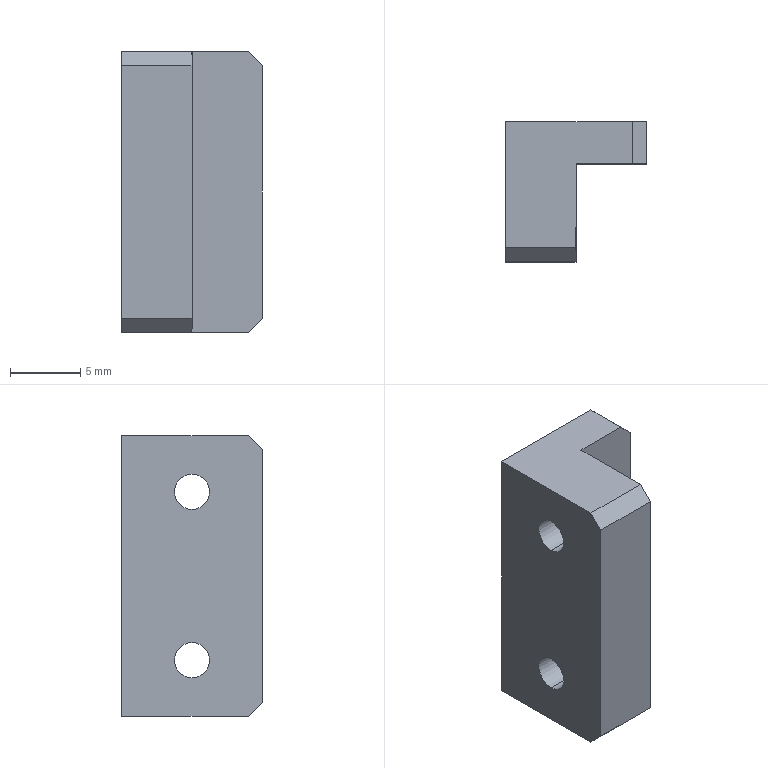Part | STEP file | FBDS-TL-002 | 1 solid | 16 faces | box 10 x 10 x 20 mm | volume 1243 mm3 | plane 12 | cylinder 4 | commonest cylinder face diameters 2.5 x4
STEP:
#1=CARTESIAN_POINT('',(5.,-5.,2.75));
#2=VERTEX_POINT('',#1);
#3=CARTESIAN_POINT('',(5.,-5.,5.25));
#4=VERTEX_POINT('',#3);
#5=CARTESIAN_POINT('',(5.,-5.,4.));
#6=DIRECTION('',(-1.,0.,0.));
#7=DIRECTION('',(0.,0.,1.));
#8=AXIS2_PLACEMENT_3D('',#5,#6,#7);
#9=CIRCLE('',#8,1.25);
#10=EDGE_CURVE('',#2,#4,#9,.T.);
#11=ORIENTED_EDGE('',*,*,#10,.F.);
#12=CARTESIAN_POINT('',(0.,-5.,2.75));
#13=VERTEX_POINT('',#12);
#14=CARTESIAN_POINT('',(0.,-5.,2.75));
#15=DIRECTION('',(-1.,0.,0.));
#16=VECTOR('',#15,1000.);
#17=LINE('',#14,#16);
#18=EDGE_CURVE('',#2,#13,#17,.T.);
#19=ORIENTED_EDGE('',*,*,#18,.T.);
#20=CARTESIAN_POINT('',(0.,-5.,5.25));
#21=VERTEX_POINT('',#20);
#22=CARTESIAN_POINT('',(0.,-5.,4.));
#23=DIRECTION('',(-1.,0.,0.));
#24=DIRECTION('',(0.,0.,1.));
#25=AXIS2_PLACEMENT_3D('',#22,#23,#24);
#26=CIRCLE('',#25,1.25);
#27=EDGE_CURVE('',#13,#21,#26,.T.);
#28=ORIENTED_EDGE('',*,*,#27,.T.);
#29=CARTESIAN_POINT('',(0.,-5.,5.25));
#30=DIRECTION('',(-1.,0.,0.));
#31=VECTOR('',#30,1000.);
#32=LINE('',#29,#31);
#33=EDGE_CURVE('',#4,#21,#32,.T.);
#34=ORIENTED_EDGE('',*,*,#33,.F.);
#35=EDGE_LOOP('',(#11,#19,#28,#34));
#36=FACE_OUTER_BOUND('',#35,.T.);
#37=CARTESIAN_POINT('',(0.,-5.,4.));
#38=DIRECTION('',(-1.,0.,0.));
#39=DIRECTION('',(0.,0.,1.));
#40=AXIS2_PLACEMENT_3D('',#37,#38,#39);
#41=CYLINDRICAL_SURFACE('',#40,1.25);
#42=ADVANCED_FACE('',(#36),#41,.F.);
#43=CARTESIAN_POINT('',(5.,-5.,14.75));
#44=VERTEX_POINT('',#43);
#45=CARTESIAN_POINT('',(5.,-5.,17.25));
#46=VERTEX_POINT('',#45);
#47=CARTESIAN_POINT('',(5.,-5.,16.));
#48=DIRECTION('',(-1.,0.,0.));
#49=DIRECTION('',(0.,0.,1.));
#50=AXIS2_PLACEMENT_3D('',#47,#48,#49);
#51=CIRCLE('',#50,1.25);
#52=EDGE_CURVE('',#44,#46,#51,.T.);
#53=ORIENTED_EDGE('',*,*,#52,.F.);
#54=CARTESIAN_POINT('',(0.,-5.,14.75));
#55=VERTEX_POINT('',#54);
#56=CARTESIAN_POINT('',(0.,-5.,14.75));
#57=DIRECTION('',(-1.,0.,0.));
#58=VECTOR('',#57,1000.);
#59=LINE('',#56,#58);
#60=EDGE_CURVE('',#44,#55,#59,.T.);
#61=ORIENTED_EDGE('',*,*,#60,.T.);
#62=CARTESIAN_POINT('',(0.,-5.,17.25));
#63=VERTEX_POINT('',#62);
#64=CARTESIAN_POINT('',(0.,-5.,16.));
#65=DIRECTION('',(-1.,0.,0.));
#66=DIRECTION('',(0.,0.,1.));
#67=AXIS2_PLACEMENT_3D('',#64,#65,#66);
#68=CIRCLE('',#67,1.25);
#69=EDGE_CURVE('',#55,#63,#68,.T.);
#70=ORIENTED_EDGE('',*,*,#69,.T.);
#71=CARTESIAN_POINT('',(0.,-5.,17.25));
#72=DIRECTION('',(-1.,0.,0.));
#73=VECTOR('',#72,1000.);
#74=LINE('',#71,#73);
#75=EDGE_CURVE('',#46,#63,#74,.T.);
#76=ORIENTED_EDGE('',*,*,#75,.F.);
#77=EDGE_LOOP('',(#53,#61,#70,#76));
#78=FACE_OUTER_BOUND('',#77,.T.);
#79=CARTESIAN_POINT('',(0.,-5.,16.));
#80=DIRECTION('',(-1.,0.,0.));
#81=DIRECTION('',(0.,0.,1.));
#82=AXIS2_PLACEMENT_3D('',#79,#80,#81);
#83=CYLINDRICAL_SURFACE('',#82,1.25);
#84=ADVANCED_FACE('',(#78),#83,.F.);
#85=CARTESIAN_POINT('',(0.,-5.,4.));
#86=DIRECTION('',(-1.,0.,0.));
#87=DIRECTION('',(0.,0.,1.));
#88=AXIS2_PLACEMENT_3D('',#85,#86,#87);
#89=CIRCLE('',#88,1.25);
#90=EDGE_CURVE('',#21,#13,#89,.T.);
#91=ORIENTED_EDGE('',*,*,#90,.F.);
#92=ORIENTED_EDGE('',*,*,#27,.F.);
#93=EDGE_LOOP('',(#91,#92));
#94=FACE_BOUND('',#93,.T.);
#95=CARTESIAN_POINT('',(0.,-5.,16.));
#96=DIRECTION('',(-1.,0.,0.));
#97=DIRECTION('',(0.,0.,1.));
#98=AXIS2_PLACEMENT_3D('',#95,#96,#97);
#99=CIRCLE('',#98,1.25);
#100=EDGE_CURVE('',#63,#55,#99,.T.);
#101=ORIENTED_EDGE('',*,*,#100,.F.);
#102=ORIENTED_EDGE('',*,*,#69,.F.);
#103=EDGE_LOOP('',(#101,#102));
#104=FACE_BOUND('',#103,.T.);
#105=CARTESIAN_POINT('',(0.,0.,0.));
#106=VERTEX_POINT('',#105);
#107=CARTESIAN_POINT('',(0.,-9.,0.));
#108=VERTEX_POINT('',#107);
#109=CARTESIAN_POINT('',(0.,-10.,0.));
#110=DIRECTION('',(0.,-1.,0.));
#111=VECTOR('',#110,1000.);
#112=LINE('',#109,#111);
#113=EDGE_CURVE('',#106,#108,#112,.T.);
#114=ORIENTED_EDGE('',*,*,#113,.T.);
#115=CARTESIAN_POINT('',(0.,-10.,1.));
#116=VERTEX_POINT('',#115);
#117=CARTESIAN_POINT('',(0.,-10.,1.));
#118=DIRECTION('',(0.,-0.7071,0.7071));
#119=VECTOR('',#118,1000.);
#120=LINE('',#117,#119);
#121=EDGE_CURVE('',#108,#116,#120,.T.);
#122=ORIENTED_EDGE('',*,*,#121,.T.);
#123=CARTESIAN_POINT('',(0.,-10.,19.));
#124=VERTEX_POINT('',#123);
#125=CARTESIAN_POINT('',(0.,-10.,20.));
#126=DIRECTION('',(0.,0.,-1.));
#127=VECTOR('',#126,1000.);
#128=LINE('',#125,#127);
#129=EDGE_CURVE('',#124,#116,#128,.T.);
#130=ORIENTED_EDGE('',*,*,#129,.F.);
#131=CARTESIAN_POINT('',(0.,-9.,20.));
#132=VERTEX_POINT('',#131);
#133=CARTESIAN_POINT('',(0.,-9.,20.));
#134=DIRECTION('',(0.,0.7071,0.7071));
#135=VECTOR('',#134,1000.);
#136=LINE('',#133,#135);
#137=EDGE_CURVE('',#124,#132,#136,.T.);
#138=ORIENTED_EDGE('',*,*,#137,.T.);
#139=CARTESIAN_POINT('',(0.,0.,20.));
#140=VERTEX_POINT('',#139);
#141=CARTESIAN_POINT('',(0.,-10.,20.));
#142=DIRECTION('',(0.,-1.,0.));
#143=VECTOR('',#142,1000.);
#144=LINE('',#141,#143);
#145=EDGE_CURVE('',#140,#132,#144,.T.);
#146=ORIENTED_EDGE('',*,*,#145,.F.);
#147=CARTESIAN_POINT('',(0.,0.,20.));
#148=DIRECTION('',(0.,0.,-1.));
#149=VECTOR('',#148,1000.);
#150=LINE('',#147,#149);
#151=EDGE_CURVE('',#140,#106,#150,.T.);
#152=ORIENTED_EDGE('',*,*,#151,.T.);
#153=EDGE_LOOP('',(#114,#122,#130,#138,#146,#152));
#154=FACE_OUTER_BOUND('',#153,.T.);
#155=CARTESIAN_POINT('',(0.,-10.,20.));
#156=DIRECTION('',(1.,0.,0.));
#157=DIRECTION('',(0.,0.,-1.));
#158=AXIS2_PLACEMENT_3D('',#155,#156,#157);
#159=PLANE('',#158);
#160=ADVANCED_FACE('',(#94,#104,#154),#159,.F.);
#161=ORIENTED_EDGE('',*,*,#129,.T.);
#162=CARTESIAN_POINT('',(5.,-10.,1.));
#163=VERTEX_POINT('',#162);
#164=CARTESIAN_POINT('',(5.,-10.,1.));
#165=DIRECTION('',(1.,0.,0.));
#166=VECTOR('',#165,1000.);
#167=LINE('',#164,#166);
#168=EDGE_CURVE('',#116,#163,#167,.T.);
#169=ORIENTED_EDGE('',*,*,#168,.T.);
#170=CARTESIAN_POINT('',(5.,-10.,19.));
#171=VERTEX_POINT('',#170);
#172=CARTESIAN_POINT('',(5.,-10.,20.));
#173=DIRECTION('',(0.,0.,-1.));
#174=VECTOR('',#173,1000.);
#175=LINE('',#172,#174);
#176=EDGE_CURVE('',#171,#163,#175,.T.);
#177=ORIENTED_EDGE('',*,*,#176,.F.);
#178=CARTESIAN_POINT('',(5.,-10.,19.));
#179=DIRECTION('',(-1.,0.,0.));
#180=VECTOR('',#179,1000.);
#181=LINE('',#178,#180);
#182=EDGE_CURVE('',#171,#124,#181,.T.);
#183=ORIENTED_EDGE('',*,*,#182,.T.);
#184=EDGE_LOOP('',(#161,#169,#177,#183));
#185=FACE_OUTER_BOUND('',#184,.T.);
#186=CARTESIAN_POINT('',(5.,-10.,20.));
#187=DIRECTION('',(0.,1.,0.));
#188=DIRECTION('',(-1.,0.,0.));
#189=AXIS2_PLACEMENT_3D('',#186,#187,#188);
#190=PLANE('',#189);
#191=ADVANCED_FACE('',(#185),#190,.F.);
#192=CARTESIAN_POINT('',(5.,-5.,4.));
#193=DIRECTION('',(-1.,0.,0.));
#194=DIRECTION('',(0.,0.,1.));
#195=AXIS2_PLACEMENT_3D('',#192,#193,#194);
#196=CIRCLE('',#195,1.25);
#197=EDGE_CURVE('',#4,#2,#196,.T.);
#198=ORIENTED_EDGE('',*,*,#197,.T.);
#199=ORIENTED_EDGE('',*,*,#10,.T.);
#200=EDGE_LOOP('',(#198,#199));
#201=FACE_BOUND('',#200,.T.);
#202=CARTESIAN_POINT('',(5.,-5.,16.));
#203=DIRECTION('',(-1.,0.,0.));
#204=DIRECTION('',(0.,0.,1.));
#205=AXIS2_PLACEMENT_3D('',#202,#203,#204);
#206=CIRCLE('',#205,1.25);
#207=EDGE_CURVE('',#46,#44,#206,.T.);
#208=ORIENTED_EDGE('',*,*,#207,.T.);
#209=ORIENTED_EDGE('',*,*,#52,.T.);
#210=EDGE_LOOP('',(#208,#209));
#211=FACE_BOUND('',#210,.T.);
#212=ORIENTED_EDGE('',*,*,#176,.T.);
#213=CARTESIAN_POINT('',(5.,-9.,0.));
#214=VERTEX_POINT('',#213);
#215=CARTESIAN_POINT('',(5.,-10.,1.));
#216=DIRECTION('',(0.,0.7071,-0.7071));
#217=VECTOR('',#216,1000.);
#218=LINE('',#215,#217);
#219=EDGE_CURVE('',#163,#214,#218,.T.);
#220=ORIENTED_EDGE('',*,*,#219,.T.);
#221=CARTESIAN_POINT('',(5.,-3.,0.));
#222=VERTEX_POINT('',#221);
#223=CARTESIAN_POINT('',(5.,-3.,0.));
#224=DIRECTION('',(0.,1.,0.));
#225=VECTOR('',#224,1000.);
#226=LINE('',#223,#225);
#227=EDGE_CURVE('',#214,#222,#226,.T.);
#228=ORIENTED_EDGE('',*,*,#227,.T.);
#229=CARTESIAN_POINT('',(5.,-3.,20.));
#230=VERTEX_POINT('',#229);
#231=CARTESIAN_POINT('',(5.,-3.,20.));
#232=DIRECTION('',(0.,0.,-1.));
#233=VECTOR('',#232,1000.);
#234=LINE('',#231,#233);
#235=EDGE_CURVE('',#230,#222,#234,.T.);
#236=ORIENTED_EDGE('',*,*,#235,.F.);
#237=CARTESIAN_POINT('',(5.,-9.,20.));
#238=VERTEX_POINT('',#237);
#239=CARTESIAN_POINT('',(5.,-3.,20.));
#240=DIRECTION('',(0.,1.,0.));
#241=VECTOR('',#240,1000.);
#242=LINE('',#239,#241);
#243=EDGE_CURVE('',#238,#230,#242,.T.);
#244=ORIENTED_EDGE('',*,*,#243,.F.);
#245=CARTESIAN_POINT('',(5.,-9.,20.));
#246=DIRECTION('',(0.,-0.7071,-0.7071));
#247=VECTOR('',#246,1000.);
#248=LINE('',#245,#247);
#249=EDGE_CURVE('',#238,#171,#248,.T.);
#250=ORIENTED_EDGE('',*,*,#249,.T.);
#251=EDGE_LOOP('',(#212,#220,#228,#236,#244,#250));
#252=FACE_OUTER_BOUND('',#251,.T.);
#253=CARTESIAN_POINT('',(5.,-3.,20.));
#254=DIRECTION('',(-1.,0.,0.));
#255=DIRECTION('',(0.,0.,1.));
#256=AXIS2_PLACEMENT_3D('',#253,#254,#255);
#257=PLANE('',#256);
#258=ADVANCED_FACE('',(#201,#211,#252),#257,.F.);
#259=CARTESIAN_POINT('',(9.,-3.,0.));
#260=VERTEX_POINT('',#259);
#261=CARTESIAN_POINT('',(10.,-3.,0.));
#262=DIRECTION('',(1.,0.,0.));
#263=VECTOR('',#262,1000.);
#264=LINE('',#261,#263);
#265=EDGE_CURVE('',#222,#260,#264,.T.);
#266=ORIENTED_EDGE('',*,*,#265,.T.);
#267=CARTESIAN_POINT('',(10.,-3.,1.));
#268=VERTEX_POINT('',#267);
#269=CARTESIAN_POINT('',(10.,-3.,1.));
#270=DIRECTION('',(0.7071,0.,0.7071));
#271=VECTOR('',#270,1000.);
#272=LINE('',#269,#271);
#273=EDGE_CURVE('',#260,#268,#272,.T.);
#274=ORIENTED_EDGE('',*,*,#273,.T.);
#275=CARTESIAN_POINT('',(10.,-3.,19.));
#276=VERTEX_POINT('',#275);
#277=CARTESIAN_POINT('',(10.,-3.,20.));
#278=DIRECTION('',(0.,0.,-1.));
#279=VECTOR('',#278,1000.);
#280=LINE('',#277,#279);
#281=EDGE_CURVE('',#276,#268,#280,.T.);
#282=ORIENTED_EDGE('',*,*,#281,.F.);
#283=CARTESIAN_POINT('',(9.,-3.,20.));
#284=VERTEX_POINT('',#283);
#285=CARTESIAN_POINT('',(9.,-3.,20.));
#286=DIRECTION('',(-0.7071,0.,0.7071));
#287=VECTOR('',#286,1000.);
#288=LINE('',#285,#287);
#289=EDGE_CURVE('',#276,#284,#288,.T.);
#290=ORIENTED_EDGE('',*,*,#289,.T.);
#291=CARTESIAN_POINT('',(10.,-3.,20.));
#292=DIRECTION('',(1.,0.,0.));
#293=VECTOR('',#292,1000.);
#294=LINE('',#291,#293);
#295=EDGE_CURVE('',#230,#284,#294,.T.);
#296=ORIENTED_EDGE('',*,*,#295,.F.);
#297=ORIENTED_EDGE('',*,*,#235,.T.);
#298=EDGE_LOOP('',(#266,#274,#282,#290,#296,#297));
#299=FACE_OUTER_BOUND('',#298,.T.);
#300=CARTESIAN_POINT('',(10.,-3.,20.));
#301=DIRECTION('',(0.,1.,0.));
#302=DIRECTION('',(-1.,0.,0.));
#303=AXIS2_PLACEMENT_3D('',#300,#301,#302);
#304=PLANE('',#303);
#305=ADVANCED_FACE('',(#299),#304,.F.);
#306=ORIENTED_EDGE('',*,*,#281,.T.);
#307=CARTESIAN_POINT('',(10.,0.,1.));
#308=VERTEX_POINT('',#307);
#309=CARTESIAN_POINT('',(10.,0.,1.));
#310=DIRECTION('',(0.,1.,0.));
#311=VECTOR('',#310,1000.);
#312=LINE('',#309,#311);
#313=EDGE_CURVE('',#268,#308,#312,.T.);
#314=ORIENTED_EDGE('',*,*,#313,.T.);
#315=CARTESIAN_POINT('',(10.,0.,19.));
#316=VERTEX_POINT('',#315);
#317=CARTESIAN_POINT('',(10.,0.,20.));
#318=DIRECTION('',(0.,0.,-1.));
#319=VECTOR('',#318,1000.);
#320=LINE('',#317,#319);
#321=EDGE_CURVE('',#316,#308,#320,.T.);
#322=ORIENTED_EDGE('',*,*,#321,.F.);
#323=CARTESIAN_POINT('',(10.,0.,19.));
#324=DIRECTION('',(0.,-1.,0.));
#325=VECTOR('',#324,1000.);
#326=LINE('',#323,#325);
#327=EDGE_CURVE('',#316,#276,#326,.T.);
#328=ORIENTED_EDGE('',*,*,#327,.T.);
#329=EDGE_LOOP('',(#306,#314,#322,#328));
#330=FACE_OUTER_BOUND('',#329,.T.);
#331=CARTESIAN_POINT('',(10.,0.,20.));
#332=DIRECTION('',(-1.,0.,0.));
#333=DIRECTION('',(0.,0.,1.));
#334=AXIS2_PLACEMENT_3D('',#331,#332,#333);
#335=PLANE('',#334);
#336=ADVANCED_FACE('',(#330),#335,.F.);
#337=ORIENTED_EDGE('',*,*,#321,.T.);
#338=CARTESIAN_POINT('',(9.,0.,0.));
#339=VERTEX_POINT('',#338);
#340=CARTESIAN_POINT('',(10.,0.,1.));
#341=DIRECTION('',(-0.7071,0.,-0.7071));
#342=VECTOR('',#341,1000.);
#343=LINE('',#340,#342);
#344=EDGE_CURVE('',#308,#339,#343,.T.);
#345=ORIENTED_EDGE('',*,*,#344,.T.);
#346=CARTESIAN_POINT('',(0.,0.,0.));
#347=DIRECTION('',(-1.,0.,0.));
#348=VECTOR('',#347,1000.);
#349=LINE('',#346,#348);
#350=EDGE_CURVE('',#339,#106,#349,.T.);
#351=ORIENTED_EDGE('',*,*,#350,.T.);
#352=ORIENTED_EDGE('',*,*,#151,.F.);
#353=CARTESIAN_POINT('',(9.,0.,20.));
#354=VERTEX_POINT('',#353);
#355=CARTESIAN_POINT('',(0.,0.,20.));
#356=DIRECTION('',(-1.,0.,0.));
#357=VECTOR('',#356,1000.);
#358=LINE('',#355,#357);
#359=EDGE_CURVE('',#354,#140,#358,.T.);
#360=ORIENTED_EDGE('',*,*,#359,.F.);
#361=CARTESIAN_POINT('',(9.,0.,20.));
#362=DIRECTION('',(0.7071,0.,-0.7071));
#363=VECTOR('',#362,1000.);
#364=LINE('',#361,#363);
#365=EDGE_CURVE('',#354,#316,#364,.T.);
#366=ORIENTED_EDGE('',*,*,#365,.T.);
#367=EDGE_LOOP('',(#337,#345,#351,#352,#360,#366));
#368=FACE_OUTER_BOUND('',#367,.T.);
#369=CARTESIAN_POINT('',(0.,0.,20.));
#370=DIRECTION('',(0.,-1.,0.));
#371=DIRECTION('',(0.,0.,-1.));
#372=AXIS2_PLACEMENT_3D('',#369,#370,#371);
#373=PLANE('',#372);
#374=ADVANCED_FACE('',(#368),#373,.F.);
#375=ORIENTED_EDGE('',*,*,#295,.T.);
#376=CARTESIAN_POINT('',(9.,0.,20.));
#377=DIRECTION('',(0.,1.,0.));
#378=VECTOR('',#377,1000.);
#379=LINE('',#376,#378);
#380=EDGE_CURVE('',#284,#354,#379,.T.);
#381=ORIENTED_EDGE('',*,*,#380,.T.);
#382=ORIENTED_EDGE('',*,*,#359,.T.);
#383=ORIENTED_EDGE('',*,*,#145,.T.);
#384=CARTESIAN_POINT('',(0.,-9.,20.));
#385=DIRECTION('',(1.,0.,0.));
#386=VECTOR('',#385,1000.);
#387=LINE('',#384,#386);
#388=EDGE_CURVE('',#132,#238,#387,.T.);
#389=ORIENTED_EDGE('',*,*,#388,.T.);
#390=ORIENTED_EDGE('',*,*,#243,.T.);
#391=EDGE_LOOP('',(#375,#381,#382,#383,#389,#390));
#392=FACE_OUTER_BOUND('',#391,.T.);
#393=CARTESIAN_POINT('',(0.,0.,20.));
#394=DIRECTION('',(0.,0.,-1.));
#395=DIRECTION('',(-1.,0.,0.));
#396=AXIS2_PLACEMENT_3D('',#393,#394,#395);
#397=PLANE('',#396);
#398=ADVANCED_FACE('',(#392),#397,.F.);
#399=ORIENTED_EDGE('',*,*,#227,.F.);
#400=CARTESIAN_POINT('',(0.,-9.,0.));
#401=DIRECTION('',(-1.,0.,0.));
#402=VECTOR('',#401,1000.);
#403=LINE('',#400,#402);
#404=EDGE_CURVE('',#214,#108,#403,.T.);
#405=ORIENTED_EDGE('',*,*,#404,.T.);
#406=ORIENTED_EDGE('',*,*,#113,.F.);
#407=ORIENTED_EDGE('',*,*,#350,.F.);
#408=CARTESIAN_POINT('',(9.,-3.,0.));
#409=DIRECTION('',(0.,-1.,0.));
#410=VECTOR('',#409,1000.);
#411=LINE('',#408,#410);
#412=EDGE_CURVE('',#339,#260,#411,.T.);
#413=ORIENTED_EDGE('',*,*,#412,.T.);
#414=ORIENTED_EDGE('',*,*,#265,.F.);
#415=EDGE_LOOP('',(#399,#405,#406,#407,#413,#414));
#416=FACE_OUTER_BOUND('',#415,.T.);
#417=CARTESIAN_POINT('',(0.,0.,0.));
#418=DIRECTION('',(0.,0.,-1.));
#419=DIRECTION('',(-1.,0.,0.));
#420=AXIS2_PLACEMENT_3D('',#417,#418,#419);
#421=PLANE('',#420);
#422=ADVANCED_FACE('',(#416),#421,.T.);
#423=ORIENTED_EDGE('',*,*,#60,.F.);
#424=ORIENTED_EDGE('',*,*,#207,.F.);
#425=ORIENTED_EDGE('',*,*,#75,.T.);
#426=ORIENTED_EDGE('',*,*,#100,.T.);
#427=EDGE_LOOP('',(#423,#424,#425,#426));
#428=FACE_OUTER_BOUND('',#427,.T.);
#429=CARTESIAN_POINT('',(0.,-5.,16.));
#430=DIRECTION('',(-1.,0.,0.));
#431=DIRECTION('',(0.,0.,1.));
#432=AXIS2_PLACEMENT_3D('',#429,#430,#431);
#433=CYLINDRICAL_SURFACE('',#432,1.25);
#434=ADVANCED_FACE('',(#428),#433,.F.);
#435=ORIENTED_EDGE('',*,*,#18,.F.);
#436=ORIENTED_EDGE('',*,*,#197,.F.);
#437=ORIENTED_EDGE('',*,*,#33,.T.);
#438=ORIENTED_EDGE('',*,*,#90,.T.);
#439=EDGE_LOOP('',(#435,#436,#437,#438));
#440=FACE_OUTER_BOUND('',#439,.T.);
#441=CARTESIAN_POINT('',(0.,-5.,4.));
#442=DIRECTION('',(-1.,0.,0.));
#443=DIRECTION('',(0.,0.,1.));
#444=AXIS2_PLACEMENT_3D('',#441,#442,#443);
#445=CYLINDRICAL_SURFACE('',#444,1.25);
#446=ADVANCED_FACE('',(#440),#445,.F.);
#447=ORIENTED_EDGE('',*,*,#121,.F.);
#448=ORIENTED_EDGE('',*,*,#404,.F.);
#449=ORIENTED_EDGE('',*,*,#219,.F.);
#450=ORIENTED_EDGE('',*,*,#168,.F.);
#451=EDGE_LOOP('',(#447,#448,#449,#450));
#452=FACE_OUTER_BOUND('',#451,.T.);
#453=CARTESIAN_POINT('',(5.,-10.,1.));
#454=DIRECTION('',(0.,-0.7071,-0.7071));
#455=DIRECTION('',(-1.,0.,0.));
#456=AXIS2_PLACEMENT_3D('',#453,#454,#455);
#457=PLANE('',#456);
#458=ADVANCED_FACE('',(#452),#457,.T.);
#459=ORIENTED_EDGE('',*,*,#273,.F.);
#460=ORIENTED_EDGE('',*,*,#412,.F.);
#461=ORIENTED_EDGE('',*,*,#344,.F.);
#462=ORIENTED_EDGE('',*,*,#313,.F.);
#463=EDGE_LOOP('',(#459,#460,#461,#462));
#464=FACE_OUTER_BOUND('',#463,.T.);
#465=CARTESIAN_POINT('',(10.,0.,1.));
#466=DIRECTION('',(0.7071,0.,-0.7071));
#467=DIRECTION('',(0.,-1.,0.));
#468=AXIS2_PLACEMENT_3D('',#465,#466,#467);
#469=PLANE('',#468);
#470=ADVANCED_FACE('',(#464),#469,.T.);
#471=ORIENTED_EDGE('',*,*,#289,.F.);
#472=ORIENTED_EDGE('',*,*,#327,.F.);
#473=ORIENTED_EDGE('',*,*,#365,.F.);
#474=ORIENTED_EDGE('',*,*,#380,.F.);
#475=EDGE_LOOP('',(#471,#472,#473,#474));
#476=FACE_OUTER_BOUND('',#475,.T.);
#477=CARTESIAN_POINT('',(9.,0.,20.));
#478=DIRECTION('',(-0.7071,0.,-0.7071));
#479=DIRECTION('',(0.,1.,0.));
#480=AXIS2_PLACEMENT_3D('',#477,#478,#479);
#481=PLANE('',#480);
#482=ADVANCED_FACE('',(#476),#481,.F.);
#483=ORIENTED_EDGE('',*,*,#137,.F.);
#484=ORIENTED_EDGE('',*,*,#182,.F.);
#485=ORIENTED_EDGE('',*,*,#249,.F.);
#486=ORIENTED_EDGE('',*,*,#388,.F.);
#487=EDGE_LOOP('',(#483,#484,#485,#486));
#488=FACE_OUTER_BOUND('',#487,.T.);
#489=CARTESIAN_POINT('',(0.,-9.,20.));
#490=DIRECTION('',(0.,0.7071,-0.7071));
#491=DIRECTION('',(1.,0.,0.));
#492=AXIS2_PLACEMENT_3D('',#489,#490,#491);
#493=PLANE('',#492);
#494=ADVANCED_FACE('',(#488),#493,.F.);
#495=CLOSED_SHELL('',(#42,#84,#160,#191,#258,#305,#336,#374,#398,#422,#434,#446,#458,#470,#482,#494));
#496=MANIFOLD_SOLID_BREP('',#495);
#497=CARTESIAN_POINT('',(0.,0.,0.));
#498=DIRECTION('',(0.,0.,1.));
#499=DIRECTION('',(1.,0.,0.));
#500=AXIS2_PLACEMENT_3D('',#497,#498,#499);
#501=(LENGTH_UNIT()NAMED_UNIT(*)SI_UNIT(.MILLI.,.METRE.));
#502=UNCERTAINTY_MEASURE_WITH_UNIT(LENGTH_MEASURE(0.00001),#501,'','');
#503=(NAMED_UNIT(*)PLANE_ANGLE_UNIT()SI_UNIT($,.RADIAN.));
#504=(NAMED_UNIT(*)SI_UNIT($,.STERADIAN.)SOLID_ANGLE_UNIT());
#505=(GEOMETRIC_REPRESENTATION_CONTEXT(3)GLOBAL_UNCERTAINTY_ASSIGNED_CONTEXT((#502))GLOBAL_UNIT_ASSIGNED_CONTEXT((#501,#503,#504))REPRESENTATION_CONTEXT('',''));
#506=ADVANCED_BREP_SHAPE_REPRESENTATION('',(#496,#500),#505);